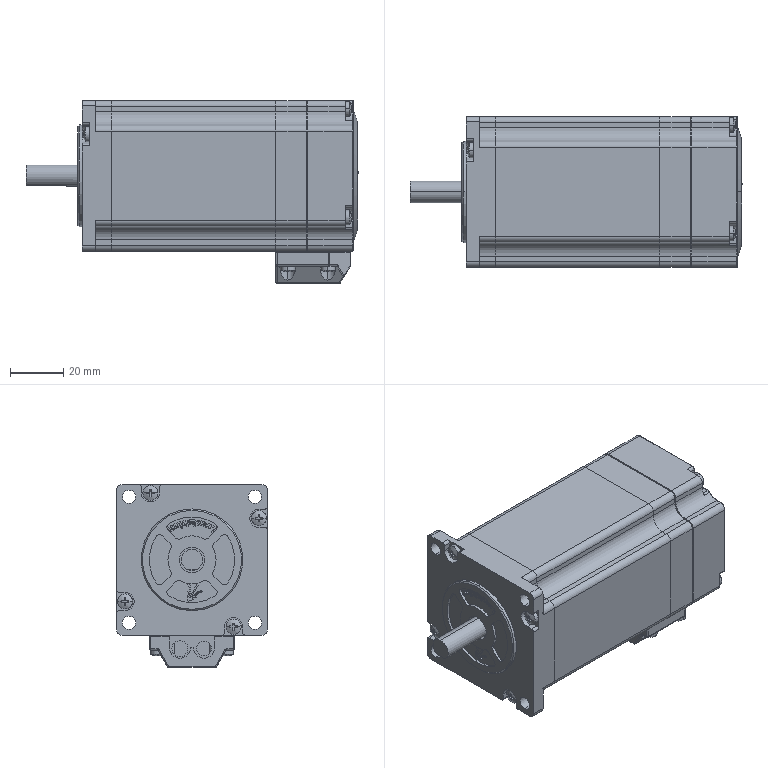Part | SolidWorks | features BaseBody 32 | 32 solids | 3195 faces | volume 141786 mm3 | plane 1460 | cylinder 996 | spline 482 | cone 257 | commonest cylinder face diameters 3 x176 0.6 x113 1 x92 2 x85 34.8 x52 4.6 x40